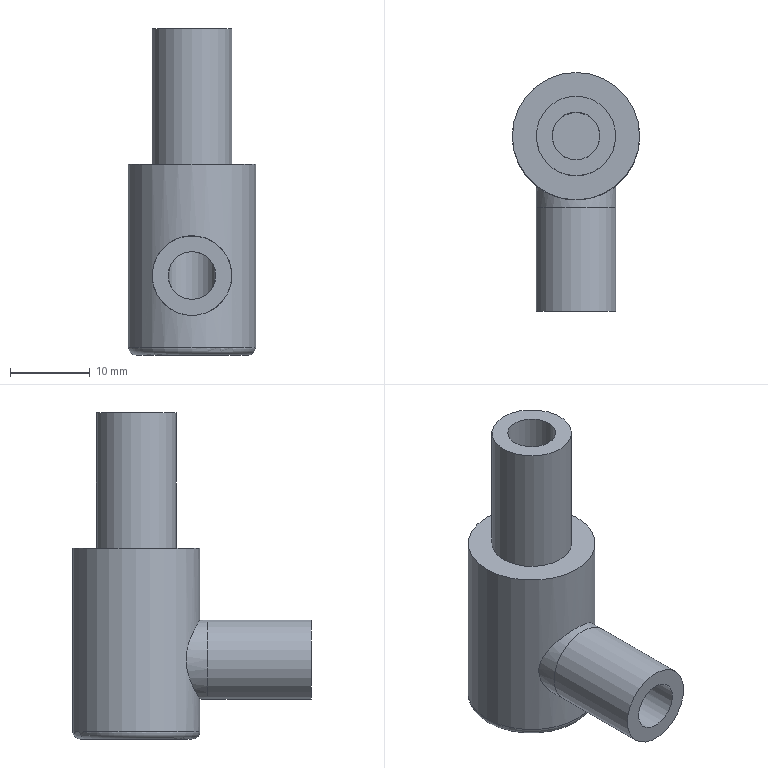Part | STEP file | 1-51.1 | 1 solid | 12 faces | box 16 x 30 x 41 mm | volume 5743 mm3 | cylinder 6 | plane 5 | torus 1 | commonest cylinder face diameters 10 x3 6 x2 16 x1
STEP:
#1=CARTESIAN_POINT('',(0.,0.,0.));
#2=DIRECTION('',(0.,0.,1.));
#3=DIRECTION('',(1.,0.,0.));
#4=AXIS2_PLACEMENT_3D('',#1,#2,#3);
#5=CARTESIAN_POINT('',(0.,8.,0.));
#6=VERTEX_POINT('',#5);
#7=CARTESIAN_POINT('',(0.,0.,0.));
#8=DIRECTION('',(0.,0.,1.));
#9=DIRECTION('',(0.,1.,0.));
#10=AXIS2_PLACEMENT_3D('',#7,#8,#9);
#11=CIRCLE('',#10,8.);
#12=CARTESIAN_POINT('',(0.,-2.144,0.));
#13=DIRECTION('',(0.,0.,1.));
#14=DIRECTION('',(1.,0.,0.));
#15=AXIS2_PLACEMENT_3D('',#12,#13,#14);
#16=PLANE('',#15);
#17=CARTESIAN_POINT('',(0.,2.144));
#18=DIRECTION('',(0.,1.));
#19=AXIS2_PLACEMENT_2D('',#17,#18);
#20=CIRCLE('',#19,8.);
#21=(GEOMETRIC_REPRESENTATION_CONTEXT(2)PARAMETRIC_REPRESENTATION_CONTEXT()REPRESENTATION_CONTEXT('',''));
#22=DEFINITIONAL_REPRESENTATION('',(#20),#21);
#23=PCURVE('',#16,#22);
#24=CARTESIAN_POINT('',(0.,0.,0.));
#25=DIRECTION('',(0.,0.,-1.));
#26=DIRECTION('',(0.,1.,0.));
#27=AXIS2_PLACEMENT_3D('',#24,#25,#26);
#28=CYLINDRICAL_SURFACE('',#27,8.);
#29=CARTESIAN_POINT('',(6.283,0.));
#30=DIRECTION('',(-1.,0.));
#31=VECTOR('',#30,1.);
#32=LINE('',#29,#31);
#33=(GEOMETRIC_REPRESENTATION_CONTEXT(2)PARAMETRIC_REPRESENTATION_CONTEXT()REPRESENTATION_CONTEXT('',''));
#34=DEFINITIONAL_REPRESENTATION('',(#32),#33);
#35=PCURVE('',#28,#34);
#36=SURFACE_CURVE('',#11,(#23,#35),.PCURVE_S1.);
#37=EDGE_CURVE('',#6,#6,#36,.T.);
#38=ORIENTED_EDGE('',*,*,#37,.T.);
#39=EDGE_LOOP('',(#38));
#40=FACE_BOUND('',#39,.T.);
#41=CARTESIAN_POINT('',(0.,5.,0.));
#42=VERTEX_POINT('',#41);
#43=CARTESIAN_POINT('',(0.,0.,0.));
#44=DIRECTION('',(0.,0.,1.));
#45=DIRECTION('',(0.,1.,0.));
#46=AXIS2_PLACEMENT_3D('',#43,#44,#45);
#47=CIRCLE('',#46,5.);
#48=CARTESIAN_POINT('',(0.,2.144));
#49=DIRECTION('',(0.,1.));
#50=AXIS2_PLACEMENT_2D('',#48,#49);
#51=CIRCLE('',#50,5.);
#52=(GEOMETRIC_REPRESENTATION_CONTEXT(2)PARAMETRIC_REPRESENTATION_CONTEXT()REPRESENTATION_CONTEXT('',''));
#53=DEFINITIONAL_REPRESENTATION('',(#51),#52);
#54=PCURVE('',#16,#53);
#55=CARTESIAN_POINT('',(0.,0.,0.));
#56=DIRECTION('',(0.,0.,1.));
#57=DIRECTION('',(0.,1.,0.));
#58=AXIS2_PLACEMENT_3D('',#55,#56,#57);
#59=CYLINDRICAL_SURFACE('',#58,5.);
#60=CARTESIAN_POINT('',(0.,0.));
#61=DIRECTION('',(1.,0.));
#62=VECTOR('',#61,1.);
#63=LINE('',#60,#62);
#64=(GEOMETRIC_REPRESENTATION_CONTEXT(2)PARAMETRIC_REPRESENTATION_CONTEXT()REPRESENTATION_CONTEXT('',''));
#65=DEFINITIONAL_REPRESENTATION('',(#63),#64);
#66=PCURVE('',#59,#65);
#67=SURFACE_CURVE('',#47,(#54,#66),.PCURVE_S1.);
#68=EDGE_CURVE('',#42,#42,#67,.T.);
#69=ORIENTED_EDGE('',*,*,#68,.F.);
#70=EDGE_LOOP('',(#69));
#71=FACE_BOUND('',#70,.T.);
#72=ADVANCED_FACE('',(#40,#71),#16,.T.);
#73=ORIENTED_EDGE('',*,*,#68,.T.);
#74=CARTESIAN_POINT('',(0.,5.,17.));
#75=VERTEX_POINT('',#74);
#76=CARTESIAN_POINT('',(0.,5.,0.));
#77=DIRECTION('',(0.,0.,1.));
#78=VECTOR('',#77,1.);
#79=LINE('',#76,#78);
#80=CARTESIAN_POINT('',(6.283,0.));
#81=DIRECTION('',(0.,1.));
#82=VECTOR('',#81,1.);
#83=LINE('',#80,#82);
#84=(GEOMETRIC_REPRESENTATION_CONTEXT(2)PARAMETRIC_REPRESENTATION_CONTEXT()REPRESENTATION_CONTEXT('',''));
#85=DEFINITIONAL_REPRESENTATION('',(#83),#84);
#86=PCURVE('',#59,#85);
#87=CARTESIAN_POINT('',(0.,0.));
#88=DIRECTION('',(0.,1.));
#89=VECTOR('',#88,1.);
#90=LINE('',#87,#89);
#91=(GEOMETRIC_REPRESENTATION_CONTEXT(2)PARAMETRIC_REPRESENTATION_CONTEXT()REPRESENTATION_CONTEXT('',''));
#92=DEFINITIONAL_REPRESENTATION('',(#90),#91);
#93=PCURVE('',#59,#92);
#94=SEAM_CURVE('',#79,(#86,#93),.PCURVE_S1.);
#95=EDGE_CURVE('',#42,#75,#94,.T.);
#96=ORIENTED_EDGE('',*,*,#95,.T.);
#97=CARTESIAN_POINT('',(0.,0.,17.));
#98=DIRECTION('',(0.,0.,1.));
#99=DIRECTION('',(0.,1.,0.));
#100=AXIS2_PLACEMENT_3D('',#97,#98,#99);
#101=CIRCLE('',#100,5.);
#102=CARTESIAN_POINT('',(0.,17.));
#103=DIRECTION('',(1.,0.));
#104=VECTOR('',#103,1.);
#105=LINE('',#102,#104);
#106=(GEOMETRIC_REPRESENTATION_CONTEXT(2)PARAMETRIC_REPRESENTATION_CONTEXT()REPRESENTATION_CONTEXT('',''));
#107=DEFINITIONAL_REPRESENTATION('',(#105),#106);
#108=PCURVE('',#59,#107);
#109=CARTESIAN_POINT('',(0.,-1.34,17.));
#110=DIRECTION('',(0.,0.,1.));
#111=DIRECTION('',(1.,0.,0.));
#112=AXIS2_PLACEMENT_3D('',#109,#110,#111);
#113=PLANE('',#112);
#114=CARTESIAN_POINT('',(0.,1.34));
#115=DIRECTION('',(0.,1.));
#116=AXIS2_PLACEMENT_2D('',#114,#115);
#117=CIRCLE('',#116,5.);
#118=(GEOMETRIC_REPRESENTATION_CONTEXT(2)PARAMETRIC_REPRESENTATION_CONTEXT()REPRESENTATION_CONTEXT('',''));
#119=DEFINITIONAL_REPRESENTATION('',(#117),#118);
#120=PCURVE('',#113,#119);
#121=SURFACE_CURVE('',#101,(#108,#120),.PCURVE_S1.);
#122=EDGE_CURVE('',#75,#75,#121,.T.);
#123=ORIENTED_EDGE('',*,*,#122,.F.);
#124=ORIENTED_EDGE('',*,*,#95,.F.);
#125=EDGE_LOOP('',(#73,#96,#123,#124));
#126=FACE_BOUND('',#125,.T.);
#127=ADVANCED_FACE('',(#126),#59,.T.);
#128=ORIENTED_EDGE('',*,*,#122,.T.);
#129=EDGE_LOOP('',(#128));
#130=FACE_BOUND('',#129,.T.);
#131=CARTESIAN_POINT('',(0.,3.,17.));
#132=VERTEX_POINT('',#131);
#133=CARTESIAN_POINT('',(0.,0.,17.));
#134=DIRECTION('',(0.,0.,1.));
#135=DIRECTION('',(0.,1.,0.));
#136=AXIS2_PLACEMENT_3D('',#133,#134,#135);
#137=CIRCLE('',#136,3.);
#138=CARTESIAN_POINT('',(0.,1.34));
#139=DIRECTION('',(0.,1.));
#140=AXIS2_PLACEMENT_2D('',#138,#139);
#141=CIRCLE('',#140,3.);
#142=(GEOMETRIC_REPRESENTATION_CONTEXT(2)PARAMETRIC_REPRESENTATION_CONTEXT()REPRESENTATION_CONTEXT('',''));
#143=DEFINITIONAL_REPRESENTATION('',(#141),#142);
#144=PCURVE('',#113,#143);
#145=CARTESIAN_POINT('',(0.,0.,17.));
#146=DIRECTION('',(0.,0.,-1.));
#147=DIRECTION('',(0.,1.,0.));
#148=AXIS2_PLACEMENT_3D('',#145,#146,#147);
#149=CYLINDRICAL_SURFACE('',#148,3.);
#150=CARTESIAN_POINT('',(6.283,0.));
#151=DIRECTION('',(-1.,0.));
#152=VECTOR('',#151,1.);
#153=LINE('',#150,#152);
#154=(GEOMETRIC_REPRESENTATION_CONTEXT(2)PARAMETRIC_REPRESENTATION_CONTEXT()REPRESENTATION_CONTEXT('',''));
#155=DEFINITIONAL_REPRESENTATION('',(#153),#154);
#156=PCURVE('',#149,#155);
#157=SURFACE_CURVE('',#137,(#144,#156),.PCURVE_S1.);
#158=EDGE_CURVE('',#132,#132,#157,.T.);
#159=ORIENTED_EDGE('',*,*,#158,.F.);
#160=EDGE_LOOP('',(#159));
#161=FACE_BOUND('',#160,.T.);
#162=ADVANCED_FACE('',(#130,#161),#113,.T.);
#163=CARTESIAN_POINT('',(0.,3.,-18.));
#164=VERTEX_POINT('',#163);
#165=CARTESIAN_POINT('',(0.,0.,-18.));
#166=DIRECTION('',(0.,0.,1.));
#167=DIRECTION('',(0.,1.,0.));
#168=AXIS2_PLACEMENT_3D('',#165,#166,#167);
#169=CIRCLE('',#168,3.);
#170=CARTESIAN_POINT('',(0.,-0.8038,-18.));
#171=DIRECTION('',(0.,0.,1.));
#172=DIRECTION('',(0.,1.,0.));
#173=AXIS2_PLACEMENT_3D('',#170,#171,#172);
#174=PLANE('',#173);
#175=CARTESIAN_POINT('',(0.8038,0.));
#176=DIRECTION('',(1.,0.));
#177=AXIS2_PLACEMENT_2D('',#175,#176);
#178=CIRCLE('',#177,3.);
#179=(GEOMETRIC_REPRESENTATION_CONTEXT(2)PARAMETRIC_REPRESENTATION_CONTEXT()REPRESENTATION_CONTEXT('',''));
#180=DEFINITIONAL_REPRESENTATION('',(#178),#179);
#181=PCURVE('',#174,#180);
#182=CARTESIAN_POINT('',(6.283,35.));
#183=DIRECTION('',(-1.,0.));
#184=VECTOR('',#183,1.);
#185=LINE('',#182,#184);
#186=(GEOMETRIC_REPRESENTATION_CONTEXT(2)PARAMETRIC_REPRESENTATION_CONTEXT()REPRESENTATION_CONTEXT('',''));
#187=DEFINITIONAL_REPRESENTATION('',(#185),#186);
#188=PCURVE('',#149,#187);
#189=SURFACE_CURVE('',#169,(#181,#188),.PCURVE_S1.);
#190=EDGE_CURVE('',#164,#164,#189,.T.);
#191=ORIENTED_EDGE('',*,*,#190,.T.);
#192=EDGE_LOOP('',(#191));
#193=FACE_BOUND('',#192,.T.);
#194=ADVANCED_FACE('',(#193),#174,.T.);
#195=CARTESIAN_POINT('',(5.,-22.,-14.));
#196=VERTEX_POINT('',#195);
#197=CARTESIAN_POINT('',(0.,-22.,-14.));
#198=DIRECTION('',(0.,-1.,0.));
#199=DIRECTION('',(1.,0.,0.));
#200=AXIS2_PLACEMENT_3D('',#197,#198,#199);
#201=CIRCLE('',#200,5.);
#202=CARTESIAN_POINT('',(-1.34,-22.,-14.));
#203=DIRECTION('',(0.,-1.,0.));
#204=DIRECTION('',(1.,0.,0.));
#205=AXIS2_PLACEMENT_3D('',#202,#203,#204);
#206=PLANE('',#205);
#207=CARTESIAN_POINT('',(1.34,0.));
#208=DIRECTION('',(1.,0.));
#209=AXIS2_PLACEMENT_2D('',#207,#208);
#210=CIRCLE('',#209,5.);
#211=(GEOMETRIC_REPRESENTATION_CONTEXT(2)PARAMETRIC_REPRESENTATION_CONTEXT()REPRESENTATION_CONTEXT('',''));
#212=DEFINITIONAL_REPRESENTATION('',(#210),#211);
#213=PCURVE('',#206,#212);
#214=CARTESIAN_POINT('',(0.,-9.,-14.));
#215=DIRECTION('',(0.,-1.,0.));
#216=DIRECTION('',(1.,0.,0.));
#217=AXIS2_PLACEMENT_3D('',#214,#215,#216);
#218=CYLINDRICAL_SURFACE('',#217,5.);
#219=CARTESIAN_POINT('',(0.,13.));
#220=DIRECTION('',(1.,0.));
#221=VECTOR('',#220,1.);
#222=LINE('',#219,#221);
#223=(GEOMETRIC_REPRESENTATION_CONTEXT(2)PARAMETRIC_REPRESENTATION_CONTEXT()REPRESENTATION_CONTEXT('',''));
#224=DEFINITIONAL_REPRESENTATION('',(#222),#223);
#225=PCURVE('',#218,#224);
#226=SURFACE_CURVE('',#201,(#213,#225),.PCURVE_S1.);
#227=EDGE_CURVE('',#196,#196,#226,.T.);
#228=ORIENTED_EDGE('',*,*,#227,.T.);
#229=EDGE_LOOP('',(#228));
#230=FACE_BOUND('',#229,.T.);
#231=CARTESIAN_POINT('',(3.,-22.,-14.));
#232=VERTEX_POINT('',#231);
#233=CARTESIAN_POINT('',(0.,-22.,-14.));
#234=DIRECTION('',(0.,-1.,0.));
#235=DIRECTION('',(1.,0.,0.));
#236=AXIS2_PLACEMENT_3D('',#233,#234,#235);
#237=CIRCLE('',#236,3.);
#238=CARTESIAN_POINT('',(1.34,0.));
#239=DIRECTION('',(1.,0.));
#240=AXIS2_PLACEMENT_2D('',#238,#239);
#241=CIRCLE('',#240,3.);
#242=(GEOMETRIC_REPRESENTATION_CONTEXT(2)PARAMETRIC_REPRESENTATION_CONTEXT()REPRESENTATION_CONTEXT('',''));
#243=DEFINITIONAL_REPRESENTATION('',(#241),#242);
#244=PCURVE('',#206,#243);
#245=CARTESIAN_POINT('',(0.,-22.,-14.));
#246=DIRECTION('',(0.,1.,0.));
#247=DIRECTION('',(1.,0.,0.));
#248=AXIS2_PLACEMENT_3D('',#245,#246,#247);
#249=CYLINDRICAL_SURFACE('',#248,3.);
#250=CARTESIAN_POINT('',(6.283,0.));
#251=DIRECTION('',(-1.,0.));
#252=VECTOR('',#251,1.);
#253=LINE('',#250,#252);
#254=(GEOMETRIC_REPRESENTATION_CONTEXT(2)PARAMETRIC_REPRESENTATION_CONTEXT()REPRESENTATION_CONTEXT('',''));
#255=DEFINITIONAL_REPRESENTATION('',(#253),#254);
#256=PCURVE('',#249,#255);
#257=SURFACE_CURVE('',#237,(#244,#256),.PCURVE_S1.);
#258=EDGE_CURVE('',#232,#232,#257,.T.);
#259=ORIENTED_EDGE('',*,*,#258,.F.);
#260=EDGE_LOOP('',(#259));
#261=FACE_BOUND('',#260,.T.);
#262=ADVANCED_FACE('',(#230,#261),#206,.T.);
#263=CARTESIAN_POINT('',(0.,3.,17.));
#264=DIRECTION('',(0.,0.,-1.));
#265=VECTOR('',#264,1.);
#266=LINE('',#263,#265);
#267=CARTESIAN_POINT('',(6.283,0.));
#268=DIRECTION('',(0.,1.));
#269=VECTOR('',#268,1.);
#270=LINE('',#267,#269);
#271=(GEOMETRIC_REPRESENTATION_CONTEXT(2)PARAMETRIC_REPRESENTATION_CONTEXT()REPRESENTATION_CONTEXT('',''));
#272=DEFINITIONAL_REPRESENTATION('',(#270),#271);
#273=PCURVE('',#149,#272);
#274=CARTESIAN_POINT('',(0.,0.));
#275=DIRECTION('',(0.,1.));
#276=VECTOR('',#275,1.);
#277=LINE('',#274,#276);
#278=(GEOMETRIC_REPRESENTATION_CONTEXT(2)PARAMETRIC_REPRESENTATION_CONTEXT()REPRESENTATION_CONTEXT('',''));
#279=DEFINITIONAL_REPRESENTATION('',(#277),#278);
#280=PCURVE('',#149,#279);
#281=SEAM_CURVE('',#266,(#273,#280),.PCURVE_S1.);
#282=EDGE_CURVE('',#132,#164,#281,.T.);
#283=ORIENTED_EDGE('',*,*,#282,.T.);
#284=ORIENTED_EDGE('',*,*,#190,.T.);
#285=ORIENTED_EDGE('',*,*,#282,.F.);
#286=ORIENTED_EDGE('',*,*,#158,.F.);
#287=EDGE_LOOP('',(#283,#284,#285,#286));
#288=FACE_BOUND('',#287,.F.);
#289=CARTESIAN_POINT('',(-3.,0.,-14.));
#290=VERTEX_POINT('',#289);
#291=CARTESIAN_POINT('',(3.,0.,-14.));
#292=VERTEX_POINT('',#291);
#293=CARTESIAN_POINT('',(-3.,0.,-14.));
#294=CARTESIAN_POINT('',(-3.,-0.6572,-13.343));
#295=CARTESIAN_POINT('',(-2.782,-1.343,-12.657));
#296=CARTESIAN_POINT('',(-1.533,-2.854,-11.146));
#297=CARTESIAN_POINT('',(-0.1206,-3.324,-10.676));
#298=CARTESIAN_POINT('',(2.463,-2.2,-11.8));
#299=CARTESIAN_POINT('',(3.,-1.003,-12.997));
#300=CARTESIAN_POINT('',(3.,0.,-14.));
#301=B_SPLINE_CURVE_WITH_KNOTS('',3,(#293,#294,#295,#296,#297,#298,#299,#300),.UNSPECIFIED.,.F.,.F.,(4,2,2,4),(0.,0.6293,1.671,2.671),.UNSPECIFIED.);
#302=CARTESIAN_POINT('',(4.712,31.));
#303=CARTESIAN_POINT('',(4.67,30.873));
#304=CARTESIAN_POINT('',(4.585,30.617));
#305=CARTESIAN_POINT('',(4.455,30.234));
#306=CARTESIAN_POINT('',(4.322,29.856));
#307=CARTESIAN_POINT('',(4.187,29.491));
#308=CARTESIAN_POINT('',(4.048,29.144));
#309=CARTESIAN_POINT('',(3.905,28.825));
#310=CARTESIAN_POINT('',(3.761,28.55));
#311=CARTESIAN_POINT('',(3.615,28.324));
#312=CARTESIAN_POINT('',(3.468,28.151));
#313=CARTESIAN_POINT('',(3.319,28.038));
#314=CARTESIAN_POINT('',(3.169,27.989));
#315=CARTESIAN_POINT('',(3.015,28.011));
#316=CARTESIAN_POINT('',(2.858,28.106));
#317=CARTESIAN_POINT('',(2.69,28.288));
#318=CARTESIAN_POINT('',(2.53,28.531));
#319=CARTESIAN_POINT('',(2.38,28.818));
#320=CARTESIAN_POINT('',(2.235,29.142));
#321=CARTESIAN_POINT('',(2.094,29.495));
#322=CARTESIAN_POINT('',(1.957,29.866));
#323=CARTESIAN_POINT('',(1.824,30.247));
#324=CARTESIAN_POINT('',(1.695,30.629));
#325=CARTESIAN_POINT('',(1.611,30.878));
#326=CARTESIAN_POINT('',(1.571,31.));
#327=B_SPLINE_CURVE_WITH_KNOTS('',3,(#302,#303,#304,#305,#306,#307,#308,#309,#310,#311,#312,#313,#314,#315,#316,#317,#318,#319,#320,#321,#322,#323,#324,#325,#326),.UNSPECIFIED.,.F.,.F.,(4,1,1,1,1,1,1,1,1,1,1,1,1,1,1,1,1,1,1,1,1,1,4),(0.,0.1214,0.2428,0.3642,0.4856,0.607,0.7284,0.8498,0.9712,1.093,1.214,1.335,1.457,1.578,1.7,1.821,1.942,2.064,2.185,2.307,2.428,2.549,2.671),.QUASI_UNIFORM_KNOTS.);
#328=(GEOMETRIC_REPRESENTATION_CONTEXT(2)PARAMETRIC_REPRESENTATION_CONTEXT()REPRESENTATION_CONTEXT('',''));
#329=DEFINITIONAL_REPRESENTATION('',(#327),#328);
#330=PCURVE('',#149,#329);
#331=CARTESIAN_POINT('',(3.142,22.));
#332=CARTESIAN_POINT('',(3.184,21.873));
#333=CARTESIAN_POINT('',(3.269,21.617));
#334=CARTESIAN_POINT('',(3.399,21.234));
#335=CARTESIAN_POINT('',(3.532,20.856));
#336=CARTESIAN_POINT('',(3.667,20.491));
#337=CARTESIAN_POINT('',(3.806,20.144));
#338=CARTESIAN_POINT('',(3.949,19.825));
#339=CARTESIAN_POINT('',(4.093,19.55));
#340=CARTESIAN_POINT('',(4.239,19.324));
#341=CARTESIAN_POINT('',(4.386,19.151));
#342=CARTESIAN_POINT('',(4.534,19.038));
#343=CARTESIAN_POINT('',(4.685,18.989));
#344=CARTESIAN_POINT('',(4.839,19.011));
#345=CARTESIAN_POINT('',(4.996,19.106));
#346=CARTESIAN_POINT('',(5.164,19.288));
#347=CARTESIAN_POINT('',(5.324,19.531));
#348=CARTESIAN_POINT('',(5.474,19.818));
#349=CARTESIAN_POINT('',(5.619,20.142));
#350=CARTESIAN_POINT('',(5.76,20.495));
#351=CARTESIAN_POINT('',(5.897,20.866));
#352=CARTESIAN_POINT('',(6.03,21.247));
#353=CARTESIAN_POINT('',(6.159,21.629));
#354=CARTESIAN_POINT('',(6.243,21.878));
#355=CARTESIAN_POINT('',(6.283,22.));
#356=B_SPLINE_CURVE_WITH_KNOTS('',3,(#331,#332,#333,#334,#335,#336,#337,#338,#339,#340,#341,#342,#343,#344,#345,#346,#347,#348,#349,#350,#351,#352,#353,#354,#355),.UNSPECIFIED.,.F.,.F.,(4,1,1,1,1,1,1,1,1,1,1,1,1,1,1,1,1,1,1,1,1,1,4),(0.,0.1214,0.2428,0.3642,0.4856,0.607,0.7284,0.8498,0.9712,1.093,1.214,1.335,1.457,1.578,1.7,1.821,1.942,2.064,2.185,2.307,2.428,2.549,2.671),.QUASI_UNIFORM_KNOTS.);
#357=(GEOMETRIC_REPRESENTATION_CONTEXT(2)PARAMETRIC_REPRESENTATION_CONTEXT()REPRESENTATION_CONTEXT('',''));
#358=DEFINITIONAL_REPRESENTATION('',(#356),#357);
#359=PCURVE('',#249,#358);
#360=SURFACE_CURVE('',#301,(#330,#359),.PCURVE_S1.);
#361=EDGE_CURVE('',#290,#292,#360,.T.);
#362=ORIENTED_EDGE('',*,*,#361,.T.);
#363=CARTESIAN_POINT('',(3.,0.,-14.));
#364=CARTESIAN_POINT('',(3.,-0.6903,-14.69));
#365=CARTESIAN_POINT('',(2.759,-1.419,-15.419));
#366=CARTESIAN_POINT('',(1.441,-2.883,-16.883));
#367=CARTESIAN_POINT('',(0.1059,-3.285,-17.285));
#368=CARTESIAN_POINT('',(-2.446,-2.24,-16.24));
#369=CARTESIAN_POINT('',(-3.,-1.014,-15.014));
#370=CARTESIAN_POINT('',(-3.,0.,-14.));
#371=B_SPLINE_CURVE_WITH_KNOTS('',3,(#363,#364,#365,#366,#367,#368,#369,#370),.UNSPECIFIED.,.F.,.F.,(4,2,2,4),(0.,0.6357,1.585,2.585),.UNSPECIFIED.);
#372=CARTESIAN_POINT('',(1.571,31.));
#373=CARTESIAN_POINT('',(1.613,31.128));
#374=CARTESIAN_POINT('',(1.699,31.385));
#375=CARTESIAN_POINT('',(1.831,31.773));
#376=CARTESIAN_POINT('',(1.965,32.155));
#377=CARTESIAN_POINT('',(2.102,32.525));
#378=CARTESIAN_POINT('',(2.243,32.875));
#379=CARTESIAN_POINT('',(2.39,33.199));
#380=CARTESIAN_POINT('',(2.536,33.474));
#381=CARTESIAN_POINT('',(2.684,33.698));
#382=CARTESIAN_POINT('',(2.833,33.866));
#383=CARTESIAN_POINT('',(2.983,33.972));
#384=CARTESIAN_POINT('',(3.135,34.012));
#385=CARTESIAN_POINT('',(3.29,33.98));
#386=CARTESIAN_POINT('',(3.449,33.873));
#387=CARTESIAN_POINT('',(3.616,33.681));
#388=CARTESIAN_POINT('',(3.771,33.438));
#389=CARTESIAN_POINT('',(3.918,33.15));
#390=CARTESIAN_POINT('',(4.06,32.828));
#391=CARTESIAN_POINT('',(4.198,32.48));
#392=CARTESIAN_POINT('',(4.333,32.113));
#393=CARTESIAN_POINT('',(4.464,31.738));
#394=CARTESIAN_POINT('',(4.591,31.363));
#395=CARTESIAN_POINT('',(4.673,31.119));
#396=CARTESIAN_POINT('',(4.712,31.));
#397=B_SPLINE_CURVE_WITH_KNOTS('',3,(#372,#373,#374,#375,#376,#377,#378,#379,#380,#381,#382,#383,#384,#385,#386,#387,#388,#389,#390,#391,#392,#393,#394,#395,#396),.UNSPECIFIED.,.F.,.F.,(4,1,1,1,1,1,1,1,1,1,1,1,1,1,1,1,1,1,1,1,1,1,4),(0.,0.1175,0.235,0.3524,0.4699,0.5874,0.7049,0.8224,0.9399,1.057,1.175,1.292,1.41,1.527,1.645,1.762,1.88,1.997,2.115,2.232,2.35,2.467,2.585),.QUASI_UNIFORM_KNOTS.);
#398=(GEOMETRIC_REPRESENTATION_CONTEXT(2)PARAMETRIC_REPRESENTATION_CONTEXT()REPRESENTATION_CONTEXT('',''));
#399=DEFINITIONAL_REPRESENTATION('',(#397),#398);
#400=PCURVE('',#149,#399);
#401=CARTESIAN_POINT('',(0.,22.));
#402=CARTESIAN_POINT('',(0.04254,21.872));
#403=CARTESIAN_POINT('',(0.1284,21.615));
#404=CARTESIAN_POINT('',(0.2599,21.227));
#405=CARTESIAN_POINT('',(0.394,20.845));
#406=CARTESIAN_POINT('',(0.5312,20.475));
#407=CARTESIAN_POINT('',(0.6722,20.125));
#408=CARTESIAN_POINT('',(0.8187,19.801));
#409=CARTESIAN_POINT('',(0.9653,19.526));
#410=CARTESIAN_POINT('',(1.113,19.302));
#411=CARTESIAN_POINT('',(1.262,19.134));
#412=CARTESIAN_POINT('',(1.412,19.028));
#413=CARTESIAN_POINT('',(1.564,18.988));
#414=CARTESIAN_POINT('',(1.719,19.02));
#415=CARTESIAN_POINT('',(1.878,19.127));
#416=CARTESIAN_POINT('',(2.045,19.319));
#417=CARTESIAN_POINT('',(2.2,19.562));
#418=CARTESIAN_POINT('',(2.348,19.85));
#419=CARTESIAN_POINT('',(2.49,20.172));
#420=CARTESIAN_POINT('',(2.628,20.52));
#421=CARTESIAN_POINT('',(2.762,20.887));
#422=CARTESIAN_POINT('',(2.893,21.262));
#423=CARTESIAN_POINT('',(3.02,21.637));
#424=CARTESIAN_POINT('',(3.102,21.881));
#425=CARTESIAN_POINT('',(3.142,22.));
#426=B_SPLINE_CURVE_WITH_KNOTS('',3,(#401,#402,#403,#404,#405,#406,#407,#408,#409,#410,#411,#412,#413,#414,#415,#416,#417,#418,#419,#420,#421,#422,#423,#424,#425),.UNSPECIFIED.,.F.,.F.,(4,1,1,1,1,1,1,1,1,1,1,1,1,1,1,1,1,1,1,1,1,1,4),(0.,0.1175,0.235,0.3524,0.4699,0.5874,0.7049,0.8224,0.9399,1.057,1.175,1.292,1.41,1.527,1.645,1.762,1.88,1.997,2.115,2.232,2.35,2.467,2.585),.QUASI_UNIFORM_KNOTS.);
#427=(GEOMETRIC_REPRESENTATION_CONTEXT(2)PARAMETRIC_REPRESENTATION_CONTEXT()REPRESENTATION_CONTEXT('',''));
#428=DEFINITIONAL_REPRESENTATION('',(#426),#427);
#429=PCURVE('',#249,#428);
#430=SURFACE_CURVE('',#371,(#400,#429),.PCURVE_S1.);
#431=EDGE_CURVE('',#292,#290,#430,.T.);
#432=ORIENTED_EDGE('',*,*,#431,.T.);
#433=EDGE_LOOP('',(#362,#432));
#434=FACE_BOUND('',#433,.F.);
#435=ADVANCED_FACE('',(#288,#434),#149,.F.);
#436=CARTESIAN_POINT('',(3.,-22.,-14.));
#437=DIRECTION('',(0.,1.,0.));
#438=VECTOR('',#437,1.);
#439=LINE('',#436,#438);
#440=CARTESIAN_POINT('',(6.283,0.));
#441=DIRECTION('',(0.,1.));
#442=VECTOR('',#441,1.);
#443=LINE('',#440,#442);
#444=(GEOMETRIC_REPRESENTATION_CONTEXT(2)PARAMETRIC_REPRESENTATION_CONTEXT()REPRESENTATION_CONTEXT('',''));
#445=DEFINITIONAL_REPRESENTATION('',(#443),#444);
#446=PCURVE('',#249,#445);
#447=CARTESIAN_POINT('',(0.,0.));
#448=DIRECTION('',(0.,1.));
#449=VECTOR('',#448,1.);
#450=LINE('',#447,#449);
#451=(GEOMETRIC_REPRESENTATION_CONTEXT(2)PARAMETRIC_REPRESENTATION_CONTEXT()REPRESENTATION_CONTEXT('',''));
#452=DEFINITIONAL_REPRESENTATION('',(#450),#451);
#453=PCURVE('',#249,#452);
#454=SEAM_CURVE('',#439,(#446,#453),.PCURVE_S1.);
#455=EDGE_CURVE('',#232,#292,#454,.T.);
#456=ORIENTED_EDGE('',*,*,#455,.T.);
#457=ORIENTED_EDGE('',*,*,#361,.F.);
#458=ORIENTED_EDGE('',*,*,#431,.F.);
#459=ORIENTED_EDGE('',*,*,#455,.F.);
#460=ORIENTED_EDGE('',*,*,#258,.F.);
#461=EDGE_LOOP('',(#456,#457,#458,#459,#460));
#462=FACE_BOUND('',#461,.F.);
#463=ADVANCED_FACE('',(#462),#249,.F.);
#464=CARTESIAN_POINT('',(5.,-6.245,-14.));
#465=VERTEX_POINT('',#464);
#466=CARTESIAN_POINT('',(5.,-6.245,-14.));
#467=CARTESIAN_POINT('',(5.,-6.245,-13.655));
#468=CARTESIAN_POINT('',(4.893,-6.331,-12.621));
#469=CARTESIAN_POINT('',(4.473,-6.646,-11.677));
#470=CARTESIAN_POINT('',(3.424,-7.274,-10.163));
#471=CARTESIAN_POINT('',(2.389,-7.736,-9.428));
#472=CARTESIAN_POINT('',(-0.05454,-8.092,-8.848));
#473=CARTESIAN_POINT('',(-1.289,-7.974,-9.02));
#474=CARTESIAN_POINT('',(-3.934,-7.159,-10.433));
#475=CARTESIAN_POINT('',(-5.,-6.245,-12.101));
#476=CARTESIAN_POINT('',(-5.,-6.245,-15.68));
#477=CARTESIAN_POINT('',(-4.167,-6.965,-17.177));
#478=CARTESIAN_POINT('',(-1.897,-7.844,-18.783));
#479=CARTESIAN_POINT('',(-0.6779,-8.07,-19.113));
#480=CARTESIAN_POINT('',(1.832,-7.888,-18.82));
#481=CARTESIAN_POINT('',(2.927,-7.498,-18.222));
#482=CARTESIAN_POINT('',(4.226,-6.817,-16.778));
#483=CARTESIAN_POINT('',(4.843,-6.371,-15.672));
#484=CARTESIAN_POINT('',(5.,-6.245,-14.418));
#485=CARTESIAN_POINT('',(5.,-6.245,-14.));
#486=B_SPLINE_CURVE_WITH_KNOTS('',3,(#466,#467,#468,#469,#470,#471,#472,#473,#474,#475,#476,#477,#478,#479,#480,#481,#482,#483,#484,#485),.UNSPECIFIED.,.T.,.F.,(1,3,1,2,2,2,2,2,2,2,1,3,1),(-0.3333,0.,0.2785,0.8356,1.887,2.915,4.436,5.782,6.823,7.857,8.524,8.857,9.135),.UNSPECIFIED.);
#487=CARTESIAN_POINT('',(0.,0.,-14.));
#488=DIRECTION('',(0.,-1.,0.));
#489=DIRECTION('',(1.,0.,0.));
#490=AXIS2_PLACEMENT_3D('',#487,#488,#489);
#491=CYLINDRICAL_SURFACE('',#490,5.);
#492=CARTESIAN_POINT('',(0.,6.245));
#493=CARTESIAN_POINT('',(0.04982,6.244));
#494=CARTESIAN_POINT('',(0.1495,6.275));
#495=CARTESIAN_POINT('',(0.2977,6.403));
#496=CARTESIAN_POINT('',(0.4438,6.597));
#497=CARTESIAN_POINT('',(0.5857,6.826));
#498=CARTESIAN_POINT('',(0.7231,7.067));
#499=CARTESIAN_POINT('',(0.8615,7.307));
#500=CARTESIAN_POINT('',(1.,7.532));
#501=CARTESIAN_POINT('',(1.141,7.729));
#502=CARTESIAN_POINT('',(1.283,7.883));
#503=CARTESIAN_POINT('',(1.429,7.979));
#504=CARTESIAN_POINT('',(1.572,8.008));
#505=CARTESIAN_POINT('',(1.712,7.976));
#506=CARTESIAN_POINT('',(1.852,7.885));
#507=CARTESIAN_POINT('',(1.993,7.741));
#508=CARTESIAN_POINT('',(2.135,7.546));
#509=CARTESIAN_POINT('',(2.276,7.314));
#510=CARTESIAN_POINT('',(2.417,7.066));
#511=CARTESIAN_POINT('',(2.558,6.82));
#512=CARTESIAN_POINT('',(2.699,6.594));
#513=CARTESIAN_POINT('',(2.842,6.408));
#514=CARTESIAN_POINT('',(2.987,6.28));
#515=CARTESIAN_POINT('',(3.136,6.229));
#516=CARTESIAN_POINT('',(3.286,6.274));
#517=CARTESIAN_POINT('',(3.43,6.397));
#518=CARTESIAN_POINT('',(3.573,6.58));
#519=CARTESIAN_POINT('',(3.714,6.804));
#520=CARTESIAN_POINT('',(3.855,7.049));
#521=CARTESIAN_POINT('',(3.995,7.296));
#522=CARTESIAN_POINT('',(4.136,7.527));
#523=CARTESIAN_POINT('',(4.276,7.721));
#524=CARTESIAN_POINT('',(4.416,7.871));
#525=CARTESIAN_POINT('',(4.556,7.969));
#526=CARTESIAN_POINT('',(4.698,8.01));
#527=CARTESIAN_POINT('',(4.845,7.984));
#528=CARTESIAN_POINT('',(4.99,7.89));
#529=CARTESIAN_POINT('',(5.131,7.742));
#530=CARTESIAN_POINT('',(5.27,7.552));
#531=CARTESIAN_POINT('',(5.408,7.331));
#532=CARTESIAN_POINT('',(5.546,7.094));
#533=CARTESIAN_POINT('',(5.686,6.845));
#534=CARTESIAN_POINT('',(5.832,6.605));
#535=CARTESIAN_POINT('',(5.981,6.406));
#536=CARTESIAN_POINT('',(6.132,6.276));
#537=CARTESIAN_POINT('',(6.233,6.244));
#538=CARTESIAN_POINT('',(6.283,6.245));
#539=B_SPLINE_CURVE_WITH_KNOTS('',3,(#492,#493,#494,#495,#496,#497,#498,#499,#500,#501,#502,#503,#504,#505,#506,#507,#508,#509,#510,#511,#512,#513,#514,#515,#516,#517,#518,#519,#520,#521,#522,#523,#524,#525,#526,#527,#528,#529,#530,#531,#532,#533,#534,#535,#536,#537,#538),.UNSPECIFIED.,.F.,.F.,(4,1,1,1,1,1,1,1,1,1,1,1,1,1,1,1,1,1,1,1,1,1,1,1,1,1,1,1,1,1,1,1,1,1,1,1,1,1,1,1,1,1,1,1,4),(0.,0.2013,0.4026,0.6039,0.8052,1.006,1.208,1.409,1.61,1.812,2.013,2.214,2.416,2.617,2.818,3.019,3.221,3.422,3.623,3.825,4.026,4.227,4.428,4.63,4.831,5.032,5.234,5.435,5.636,5.838,6.039,6.24,6.441,6.643,6.844,7.045,7.247,7.448,7.649,7.85,8.052,8.253,8.454,8.656,8.857),.QUASI_UNIFORM_KNOTS.);
#540=(GEOMETRIC_REPRESENTATION_CONTEXT(2)PARAMETRIC_REPRESENTATION_CONTEXT()REPRESENTATION_CONTEXT('',''));
#541=DEFINITIONAL_REPRESENTATION('',(#539),#540);
#542=PCURVE('',#491,#541);
#543=CARTESIAN_POINT('',(2.466,14.));
#544=CARTESIAN_POINT('',(2.466,13.751));
#545=CARTESIAN_POINT('',(2.472,13.253));
#546=CARTESIAN_POINT('',(2.499,12.528));
#547=CARTESIAN_POINT('',(2.54,11.846));
#548=CARTESIAN_POINT('',(2.592,11.227));
#549=CARTESIAN_POINT('',(2.653,10.681));
#550=CARTESIAN_POINT('',(2.721,10.193));
#551=CARTESIAN_POINT('',(2.796,9.777));
#552=CARTESIAN_POINT('',(2.877,9.44));
#553=CARTESIAN_POINT('',(2.963,9.188));
#554=CARTESIAN_POINT('',(3.053,9.032));
#555=CARTESIAN_POINT('',(3.142,8.982));
#556=CARTESIAN_POINT('',(3.23,9.032));
#557=CARTESIAN_POINT('',(3.317,9.18));
#558=CARTESIAN_POINT('',(3.401,9.424));
#559=CARTESIAN_POINT('',(3.483,9.761));
#560=CARTESIAN_POINT('',(3.56,10.181));
#561=CARTESIAN_POINT('',(3.63,10.675));
#562=CARTESIAN_POINT('',(3.692,11.235));
#563=CARTESIAN_POINT('',(3.744,11.853));
#564=CARTESIAN_POINT('',(3.784,12.52));
#565=CARTESIAN_POINT('',(3.81,13.226));
#566=CARTESIAN_POINT('',(3.82,13.972));
#567=CARTESIAN_POINT('',(3.811,14.72));
#568=CARTESIAN_POINT('',(3.786,15.428));
#569=CARTESIAN_POINT('',(3.747,16.098));
#570=CARTESIAN_POINT('',(3.696,16.719));
#571=CARTESIAN_POINT('',(3.635,17.282));
#572=CARTESIAN_POINT('',(3.566,17.78));
#573=CARTESIAN_POINT('',(3.49,18.205));
#574=CARTESIAN_POINT('',(3.41,18.547));
#575=CARTESIAN_POINT('',(3.326,18.799));
#576=CARTESIAN_POINT('',(3.239,18.957));
#577=CARTESIAN_POINT('',(3.151,19.018));
#578=CARTESIAN_POINT('',(3.059,18.974));
#579=CARTESIAN_POINT('',(2.969,18.826));
#580=CARTESIAN_POINT('',(2.884,18.585));
#581=CARTESIAN_POINT('',(2.804,18.257));
#582=CARTESIAN_POINT('',(2.728,17.849));
#583=CARTESIAN_POINT('',(2.659,17.373));
#584=CARTESIAN_POINT('',(2.597,16.82));
#585=CARTESIAN_POINT('',(2.542,16.185));
#586=CARTESIAN_POINT('',(2.499,15.493));
#587=CARTESIAN_POINT('',(2.473,14.757));
#588=CARTESIAN_POINT('',(2.466,14.253));
#589=CARTESIAN_POINT('',(2.466,14.));
#590=B_SPLINE_CURVE_WITH_KNOTS('',3,(#543,#544,#545,#546,#547,#548,#549,#550,#551,#552,#553,#554,#555,#556,#557,#558,#559,#560,#561,#562,#563,#564,#565,#566,#567,#568,#569,#570,#571,#572,#573,#574,#575,#576,#577,#578,#579,#580,#581,#582,#583,#584,#585,#586,#587,#588,#589),.UNSPECIFIED.,.T.,.F.,(4,1,1,1,1,1,1,1,1,1,1,1,1,1,1,1,1,1,1,1,1,1,1,1,1,1,1,1,1,1,1,1,1,1,1,1,1,1,1,1,1,1,1,1,4),(0.,0.2013,0.4026,0.6039,0.8052,1.006,1.208,1.409,1.61,1.812,2.013,2.214,2.416,2.617,2.818,3.019,3.221,3.422,3.623,3.825,4.026,4.227,4.428,4.63,4.831,5.032,5.234,5.435,5.636,5.838,6.039,6.24,6.441,6.643,6.844,7.045,7.247,7.448,7.649,7.85,8.052,8.253,8.454,8.656,8.857),.QUASI_UNIFORM_KNOTS.);
#591=(GEOMETRIC_REPRESENTATION_CONTEXT(2)PARAMETRIC_REPRESENTATION_CONTEXT()REPRESENTATION_CONTEXT('',''));
#592=DEFINITIONAL_REPRESENTATION('',(#590),#591);
#593=PCURVE('',#28,#592);
#594=SURFACE_CURVE('',#486,(#542,#593),.PCURVE_S1.);
#595=EDGE_CURVE('',#465,#465,#594,.T.);
#596=ORIENTED_EDGE('',*,*,#595,.T.);
#597=CARTESIAN_POINT('',(5.,-9.,-14.));
#598=VERTEX_POINT('',#597);
#599=CARTESIAN_POINT('',(5.,-6.245,-14.));
#600=DIRECTION('',(0.,-1.,0.));
#601=VECTOR('',#600,1.);
#602=LINE('',#599,#601);
#603=CARTESIAN_POINT('',(6.283,6.245));
#604=DIRECTION('',(0.,1.));
#605=VECTOR('',#604,1.);
#606=LINE('',#603,#605);
#607=(GEOMETRIC_REPRESENTATION_CONTEXT(2)PARAMETRIC_REPRESENTATION_CONTEXT()REPRESENTATION_CONTEXT('',''));
#608=DEFINITIONAL_REPRESENTATION('',(#606),#607);
#609=PCURVE('',#491,#608);
#610=CARTESIAN_POINT('',(0.,6.245));
#611=DIRECTION('',(0.,1.));
#612=VECTOR('',#611,1.);
#613=LINE('',#610,#612);
#614=(GEOMETRIC_REPRESENTATION_CONTEXT(2)PARAMETRIC_REPRESENTATION_CONTEXT()REPRESENTATION_CONTEXT('',''));
#615=DEFINITIONAL_REPRESENTATION('',(#613),#614);
#616=PCURVE('',#491,#615);
#617=SEAM_CURVE('',#602,(#609,#616),.PCURVE_S1.);
#618=EDGE_CURVE('',#465,#598,#617,.T.);
#619=ORIENTED_EDGE('',*,*,#618,.T.);
#620=CARTESIAN_POINT('',(0.,-9.,-14.));
#621=DIRECTION('',(0.,-1.,0.));
#622=DIRECTION('',(1.,0.,0.));
#623=AXIS2_PLACEMENT_3D('',#620,#621,#622);
#624=CIRCLE('',#623,5.);
#625=CARTESIAN_POINT('',(0.,9.));
#626=DIRECTION('',(1.,0.));
#627=VECTOR('',#626,1.);
#628=LINE('',#625,#627);
#629=(GEOMETRIC_REPRESENTATION_CONTEXT(2)PARAMETRIC_REPRESENTATION_CONTEXT()REPRESENTATION_CONTEXT('',''));
#630=DEFINITIONAL_REPRESENTATION('',(#628),#629);
#631=PCURVE('',#491,#630);
#632=CARTESIAN_POINT('',(0.,0.));
#633=DIRECTION('',(1.,0.));
#634=VECTOR('',#633,1.);
#635=LINE('',#632,#634);
#636=(GEOMETRIC_REPRESENTATION_CONTEXT(2)PARAMETRIC_REPRESENTATION_CONTEXT()REPRESENTATION_CONTEXT('',''));
#637=DEFINITIONAL_REPRESENTATION('',(#635),#636);
#638=PCURVE('',#218,#637);
#639=SURFACE_CURVE('',#624,(#631,#638),.PCURVE_S1.);
#640=EDGE_CURVE('',#598,#598,#639,.T.);
#641=ORIENTED_EDGE('',*,*,#640,.F.);
#642=ORIENTED_EDGE('',*,*,#618,.F.);
#643=EDGE_LOOP('',(#596,#619,#641,#642));
#644=FACE_BOUND('',#643,.T.);
#645=ADVANCED_FACE('',(#644),#491,.T.);
#646=ORIENTED_EDGE('',*,*,#227,.F.);
#647=CARTESIAN_POINT('',(5.,-9.,-14.));
#648=DIRECTION('',(0.,-1.,0.));
#649=VECTOR('',#648,1.);
#650=LINE('',#647,#649);
#651=CARTESIAN_POINT('',(0.,0.));
#652=DIRECTION('',(0.,1.));
#653=VECTOR('',#652,1.);
#654=LINE('',#651,#653);
#655=(GEOMETRIC_REPRESENTATION_CONTEXT(2)PARAMETRIC_REPRESENTATION_CONTEXT()REPRESENTATION_CONTEXT('',''));
#656=DEFINITIONAL_REPRESENTATION('',(#654),#655);
#657=PCURVE('',#218,#656);
#658=CARTESIAN_POINT('',(6.283,0.));
#659=DIRECTION('',(0.,1.));
#660=VECTOR('',#659,1.);
#661=LINE('',#658,#660);
#662=(GEOMETRIC_REPRESENTATION_CONTEXT(2)PARAMETRIC_REPRESENTATION_CONTEXT()REPRESENTATION_CONTEXT('',''));
#663=DEFINITIONAL_REPRESENTATION('',(#661),#662);
#664=PCURVE('',#218,#663);
#665=SEAM_CURVE('',#650,(#657,#664),.PCURVE_S1.);
#666=EDGE_CURVE('',#598,#196,#665,.T.);
#667=ORIENTED_EDGE('',*,*,#666,.F.);
#668=ORIENTED_EDGE('',*,*,#640,.T.);
#669=ORIENTED_EDGE('',*,*,#666,.T.);
#670=EDGE_LOOP('',(#646,#667,#668,#669));
#671=FACE_BOUND('',#670,.T.);
#672=ADVANCED_FACE('',(#671),#218,.T.);
#673=CARTESIAN_POINT('',(0.,7.,-24.));
#674=VERTEX_POINT('',#673);
#675=CARTESIAN_POINT('',(0.,0.,-24.));
#676=DIRECTION('',(0.,0.,1.));
#677=DIRECTION('',(0.,1.,0.));
#678=AXIS2_PLACEMENT_3D('',#675,#676,#677);
#679=CIRCLE('',#678,7.);
#680=CARTESIAN_POINT('',(0.,-2.144,-24.));
#681=DIRECTION('',(0.,0.,1.));
#682=DIRECTION('',(1.,0.,0.));
#683=AXIS2_PLACEMENT_3D('',#680,#681,#682);
#684=PLANE('',#683);
#685=CARTESIAN_POINT('',(0.,2.144));
#686=DIRECTION('',(0.,1.));
#687=AXIS2_PLACEMENT_2D('',#685,#686);
#688=CIRCLE('',#687,7.);
#689=(GEOMETRIC_REPRESENTATION_CONTEXT(2)PARAMETRIC_REPRESENTATION_CONTEXT()REPRESENTATION_CONTEXT('',''));
#690=DEFINITIONAL_REPRESENTATION('',(#688),#689);
#691=PCURVE('',#684,#690);
#692=CARTESIAN_POINT('',(0.,0.,-23.));
#693=DIRECTION('',(0.,0.,-1.));
#694=DIRECTION('',(0.,1.,0.));
#695=AXIS2_PLACEMENT_3D('',#692,#693,#694);
#696=TOROIDAL_SURFACE('',#695,7.,1.);
#697=CARTESIAN_POINT('',(6.283,1.571));
#698=DIRECTION('',(-1.,0.));
#699=VECTOR('',#698,1.);
#700=LINE('',#697,#699);
#701=(GEOMETRIC_REPRESENTATION_CONTEXT(2)PARAMETRIC_REPRESENTATION_CONTEXT()REPRESENTATION_CONTEXT('',''));
#702=DEFINITIONAL_REPRESENTATION('',(#700),#701);
#703=PCURVE('',#696,#702);
#704=SURFACE_CURVE('',#679,(#691,#703),.PCURVE_S1.);
#705=EDGE_CURVE('',#674,#674,#704,.T.);
#706=ORIENTED_EDGE('',*,*,#705,.T.);
#707=EDGE_LOOP('',(#706));
#708=FACE_BOUND('',#707,.F.);
#709=ADVANCED_FACE('',(#708),#684,.F.);
#710=CARTESIAN_POINT('',(0.,8.,-23.));
#711=VERTEX_POINT('',#710);
#712=CARTESIAN_POINT('',(0.,8.,0.));
#713=DIRECTION('',(0.,0.,-1.));
#714=VECTOR('',#713,1.);
#715=LINE('',#712,#714);
#716=CARTESIAN_POINT('',(6.283,0.));
#717=DIRECTION('',(0.,1.));
#718=VECTOR('',#717,1.);
#719=LINE('',#716,#718);
#720=(GEOMETRIC_REPRESENTATION_CONTEXT(2)PARAMETRIC_REPRESENTATION_CONTEXT()REPRESENTATION_CONTEXT('',''));
#721=DEFINITIONAL_REPRESENTATION('',(#719),#720);
#722=PCURVE('',#28,#721);
#723=CARTESIAN_POINT('',(0.,0.));
#724=DIRECTION('',(0.,1.));
#725=VECTOR('',#724,1.);
#726=LINE('',#723,#725);
#727=(GEOMETRIC_REPRESENTATION_CONTEXT(2)PARAMETRIC_REPRESENTATION_CONTEXT()REPRESENTATION_CONTEXT('',''));
#728=DEFINITIONAL_REPRESENTATION('',(#726),#727);
#729=PCURVE('',#28,#728);
#730=SEAM_CURVE('',#715,(#722,#729),.PCURVE_S1.);
#731=EDGE_CURVE('',#6,#711,#730,.T.);
#732=ORIENTED_EDGE('',*,*,#731,.T.);
#733=CARTESIAN_POINT('',(0.,0.,-23.));
#734=DIRECTION('',(0.,0.,1.));
#735=DIRECTION('',(0.,1.,0.));
#736=AXIS2_PLACEMENT_3D('',#733,#734,#735);
#737=CIRCLE('',#736,8.);
#738=CARTESIAN_POINT('',(6.283,23.));
#739=DIRECTION('',(-1.,0.));
#740=VECTOR('',#739,1.);
#741=LINE('',#738,#740);
#742=(GEOMETRIC_REPRESENTATION_CONTEXT(2)PARAMETRIC_REPRESENTATION_CONTEXT()REPRESENTATION_CONTEXT('',''));
#743=DEFINITIONAL_REPRESENTATION('',(#741),#742);
#744=PCURVE('',#28,#743);
#745=CARTESIAN_POINT('',(6.283,0.));
#746=DIRECTION('',(-1.,0.));
#747=VECTOR('',#746,1.);
#748=LINE('',#745,#747);
#749=(GEOMETRIC_REPRESENTATION_CONTEXT(2)PARAMETRIC_REPRESENTATION_CONTEXT()REPRESENTATION_CONTEXT('',''));
#750=DEFINITIONAL_REPRESENTATION('',(#748),#749);
#751=PCURVE('',#696,#750);
#752=SURFACE_CURVE('',#737,(#744,#751),.PCURVE_S1.);
#753=EDGE_CURVE('',#711,#711,#752,.T.);
#754=ORIENTED_EDGE('',*,*,#753,.T.);
#755=ORIENTED_EDGE('',*,*,#731,.F.);
#756=ORIENTED_EDGE('',*,*,#37,.F.);
#757=EDGE_LOOP('',(#732,#754,#755,#756));
#758=FACE_BOUND('',#757,.T.);
#759=ORIENTED_EDGE('',*,*,#595,.F.);
#760=EDGE_LOOP('',(#759));
#761=FACE_BOUND('',#760,.T.);
#762=ADVANCED_FACE('',(#758,#761),#28,.T.);
#763=CARTESIAN_POINT('',(0.,7.,-23.));
#764=DIRECTION('',(1.,0.,0.));
#765=DIRECTION('',(0.,0.,-1.));
#766=AXIS2_PLACEMENT_3D('',#763,#764,#765);
#767=CIRCLE('',#766,1.);
#768=CARTESIAN_POINT('',(0.,1.571));
#769=CARTESIAN_POINT('',(0.,1.547));
#770=CARTESIAN_POINT('',(0.,1.499));
#771=CARTESIAN_POINT('',(0.,1.428));
#772=CARTESIAN_POINT('',(0.,1.357));
#773=CARTESIAN_POINT('',(0.,1.285));
#774=CARTESIAN_POINT('',(0.,1.214));
#775=CARTESIAN_POINT('',(0.,1.142));
#776=CARTESIAN_POINT('',(0.,1.071));
#777=CARTESIAN_POINT('',(0.,0.9996));
#778=CARTESIAN_POINT('',(0.,0.9282));
#779=CARTESIAN_POINT('',(0.,0.8568));
#780=CARTESIAN_POINT('',(0.,0.7854));
#781=CARTESIAN_POINT('',(0.,0.714));
#782=CARTESIAN_POINT('',(0.,0.6426));
#783=CARTESIAN_POINT('',(0.,0.5712));
#784=CARTESIAN_POINT('',(0.,0.4998));
#785=CARTESIAN_POINT('',(0.,0.4284));
#786=CARTESIAN_POINT('',(0.,0.357));
#787=CARTESIAN_POINT('',(0.,0.2856));
#788=CARTESIAN_POINT('',(0.,0.2142));
#789=CARTESIAN_POINT('',(0.,0.1428));
#790=CARTESIAN_POINT('',(0.,0.0714));
#791=CARTESIAN_POINT('',(0.,0.0238));
#792=CARTESIAN_POINT('',(0.,0.));
#793=B_SPLINE_CURVE_WITH_KNOTS('',3,(#768,#769,#770,#771,#772,#773,#774,#775,#776,#777,#778,#779,#780,#781,#782,#783,#784,#785,#786,#787,#788,#789,#790,#791,#792),.UNSPECIFIED.,.F.,.F.,(4,1,1,1,1,1,1,1,1,1,1,1,1,1,1,1,1,1,1,1,1,1,4),(0.,0.0714,0.1428,0.2142,0.2856,0.357,0.4284,0.4998,0.5712,0.6426,0.714,0.7854,0.8568,0.9282,0.9996,1.071,1.142,1.214,1.285,1.357,1.428,1.499,1.571),.QUASI_UNIFORM_KNOTS.);
#794=(GEOMETRIC_REPRESENTATION_CONTEXT(2)PARAMETRIC_REPRESENTATION_CONTEXT()REPRESENTATION_CONTEXT('',''));
#795=DEFINITIONAL_REPRESENTATION('',(#793),#794);
#796=PCURVE('',#696,#795);
#797=CARTESIAN_POINT('',(6.283,1.571));
#798=CARTESIAN_POINT('',(6.283,1.547));
#799=CARTESIAN_POINT('',(6.283,1.499));
#800=CARTESIAN_POINT('',(6.283,1.428));
#801=CARTESIAN_POINT('',(6.283,1.357));
#802=CARTESIAN_POINT('',(6.283,1.285));
#803=CARTESIAN_POINT('',(6.283,1.214));
#804=CARTESIAN_POINT('',(6.283,1.142));
#805=CARTESIAN_POINT('',(6.283,1.071));
#806=CARTESIAN_POINT('',(6.283,0.9996));
#807=CARTESIAN_POINT('',(6.283,0.9282));
#808=CARTESIAN_POINT('',(6.283,0.8568));
#809=CARTESIAN_POINT('',(6.283,0.7854));
#810=CARTESIAN_POINT('',(6.283,0.714));
#811=CARTESIAN_POINT('',(6.283,0.6426));
#812=CARTESIAN_POINT('',(6.283,0.5712));
#813=CARTESIAN_POINT('',(6.283,0.4998));
#814=CARTESIAN_POINT('',(6.283,0.4284));
#815=CARTESIAN_POINT('',(6.283,0.357));
#816=CARTESIAN_POINT('',(6.283,0.2856));
#817=CARTESIAN_POINT('',(6.283,0.2142));
#818=CARTESIAN_POINT('',(6.283,0.1428));
#819=CARTESIAN_POINT('',(6.283,0.0714));
#820=CARTESIAN_POINT('',(6.283,0.0238));
#821=CARTESIAN_POINT('',(6.283,0.));
#822=B_SPLINE_CURVE_WITH_KNOTS('',3,(#797,#798,#799,#800,#801,#802,#803,#804,#805,#806,#807,#808,#809,#810,#811,#812,#813,#814,#815,#816,#817,#818,#819,#820,#821),.UNSPECIFIED.,.F.,.F.,(4,1,1,1,1,1,1,1,1,1,1,1,1,1,1,1,1,1,1,1,1,1,4),(0.,0.0714,0.1428,0.2142,0.2856,0.357,0.4284,0.4998,0.5712,0.6426,0.714,0.7854,0.8568,0.9282,0.9996,1.071,1.142,1.214,1.285,1.357,1.428,1.499,1.571),.QUASI_UNIFORM_KNOTS.);
#823=(GEOMETRIC_REPRESENTATION_CONTEXT(2)PARAMETRIC_REPRESENTATION_CONTEXT()REPRESENTATION_CONTEXT('',''));
#824=DEFINITIONAL_REPRESENTATION('',(#822),#823);
#825=PCURVE('',#696,#824);
#826=SEAM_CURVE('',#767,(#796,#825),.PCURVE_S1.);
#827=EDGE_CURVE('',#674,#711,#826,.T.);
#828=ORIENTED_EDGE('',*,*,#827,.T.);
#829=ORIENTED_EDGE('',*,*,#753,.F.);
#830=ORIENTED_EDGE('',*,*,#827,.F.);
#831=ORIENTED_EDGE('',*,*,#705,.T.);
#832=EDGE_LOOP('',(#828,#829,#830,#831));
#833=FACE_BOUND('',#832,.T.);
#834=ADVANCED_FACE('',(#833),#696,.T.);
#835=CLOSED_SHELL('',(#72,#127,#162,#194,#262,#435,#463,#645,#672,#709,#762,#834));
#836=MANIFOLD_SOLID_BREP('',#835);
#837=(LENGTH_UNIT()NAMED_UNIT(*)SI_UNIT(.MILLI.,.METRE.));
#838=UNCERTAINTY_MEASURE_WITH_UNIT(LENGTH_MEASURE(0.0005),#837,'','');
#839=(NAMED_UNIT(*)PLANE_ANGLE_UNIT()SI_UNIT($,.RADIAN.));
#840=(NAMED_UNIT(*)SI_UNIT($,.STERADIAN.)SOLID_ANGLE_UNIT());
#841=(GEOMETRIC_REPRESENTATION_CONTEXT(3)GLOBAL_UNCERTAINTY_ASSIGNED_CONTEXT((#838))GLOBAL_UNIT_ASSIGNED_CONTEXT((#837,#839,#840))REPRESENTATION_CONTEXT('',''));
#842=ADVANCED_BREP_SHAPE_REPRESENTATION('',(#4,#836),#841);